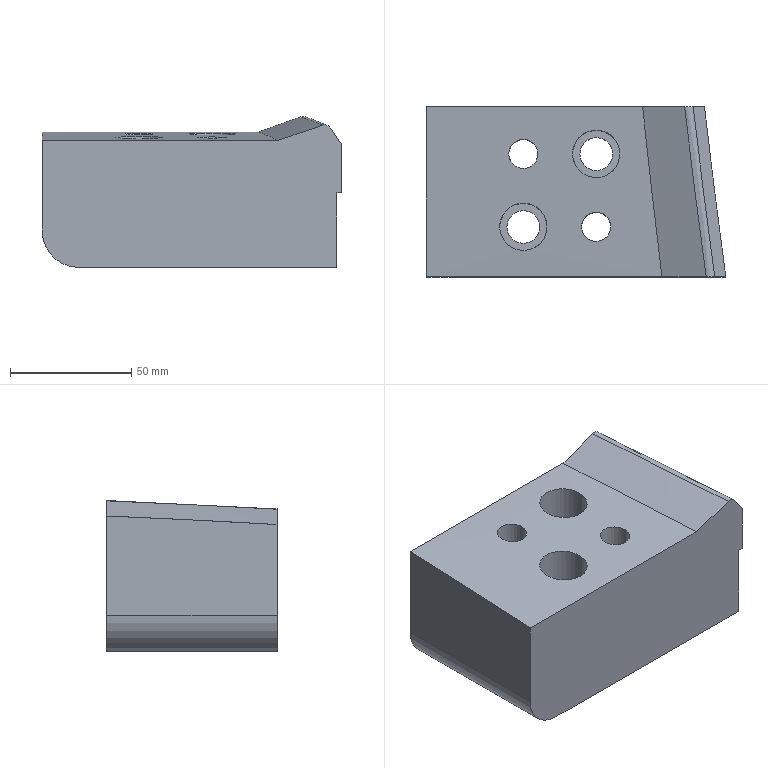Part | NX | features MAIN_BODY 2 | 1 solid | 20 faces | box 123.323 x 70 x 62.141 mm | volume 406291 mm3 | spline 7 | cylinder 7 | plane 6 | commonest cylinder face diameters 12 x2 13.5 x2 19.5 x2 30 x1
STEP:
#1=CARTESIAN_POINT('',(-841.75,-399.358,-90.));
#2=VERTEX_POINT('',#1);
#3=CARTESIAN_POINT('',(-835.,-399.358,-90.));
#4=DIRECTION('',(-0.000000341,0.00000017,-1.));
#5=DIRECTION('',(-1.,0.,0.000000341));
#6=AXIS2_PLACEMENT_3D('',#3,#4,#5);
#7=CIRCLE('',#6,6.75);
#8=EDGE_CURVE('',#2,#2,#7,.T.);
#9=ORIENTED_EDGE('',*,*,#8,.F.);
#10=EDGE_LOOP('',(#9));
#11=FACE_BOUND('',#10,.T.);
#12=CARTESIAN_POINT('',(-841.,-369.358,-90.));
#13=VERTEX_POINT('',#12);
#14=CARTESIAN_POINT('',(-835.,-369.358,-90.));
#15=DIRECTION('',(-0.000000341,0.00000017,-1.));
#16=DIRECTION('',(-1.,0.,0.000000341));
#17=AXIS2_PLACEMENT_3D('',#14,#15,#16);
#18=CIRCLE('',#17,6.);
#19=EDGE_CURVE('',#13,#13,#18,.T.);
#20=ORIENTED_EDGE('',*,*,#19,.F.);
#21=EDGE_LOOP('',(#20));
#22=FACE_BOUND('',#21,.T.);
#23=CARTESIAN_POINT('',(-811.75,-369.358,-90.));
#24=VERTEX_POINT('',#23);
#25=CARTESIAN_POINT('',(-805.,-369.358,-90.));
#26=DIRECTION('',(-0.000000341,0.00000017,-1.));
#27=DIRECTION('',(-1.,0.,0.000000341));
#28=AXIS2_PLACEMENT_3D('',#25,#26,#27);
#29=CIRCLE('',#28,6.75);
#30=EDGE_CURVE('',#24,#24,#29,.T.);
#31=ORIENTED_EDGE('',*,*,#30,.F.);
#32=EDGE_LOOP('',(#31));
#33=FACE_BOUND('',#32,.T.);
#34=CARTESIAN_POINT('',(-811.,-399.358,-90.));
#35=VERTEX_POINT('',#34);
#36=CARTESIAN_POINT('',(-805.,-399.358,-90.));
#37=DIRECTION('',(-0.000000341,0.00000017,-1.));
#38=DIRECTION('',(-1.,0.,0.000000341));
#39=AXIS2_PLACEMENT_3D('',#36,#37,#38);
#40=CIRCLE('',#39,6.);
#41=EDGE_CURVE('',#35,#35,#40,.T.);
#42=ORIENTED_EDGE('',*,*,#41,.F.);
#43=EDGE_LOOP('',(#42));
#44=FACE_BOUND('',#43,.T.);
#45=CARTESIAN_POINT('',(-860.,-350.,-90.));
#46=VERTEX_POINT('',#45);
#47=CARTESIAN_POINT('',(-762.48,-350.,-90.));
#48=VERTEX_POINT('',#47);
#49=CARTESIAN_POINT('',(-0.00003074,-350.,-90.));
#50=DIRECTION('',(-1.,0.,0.000000341));
#51=VECTOR('',#50,1000.);
#52=LINE('',#49,#51);
#53=EDGE_CURVE('',#46,#48,#52,.F.);
#54=ORIENTED_EDGE('',*,*,#53,.T.);
#55=CARTESIAN_POINT('',(-753.694,-420.,-90.));
#56=VERTEX_POINT('',#55);
#57=CARTESIAN_POINT('',(-753.694,-420.,-90.));
#58=CARTESIAN_POINT('',(-755.213,-408.34,-90.));
#59=CARTESIAN_POINT('',(-758.313,-385.028,-90.));
#60=CARTESIAN_POINT('',(-761.09,-361.676,-90.));
#61=CARTESIAN_POINT('',(-762.48,-350.,-90.));
#62=B_SPLINE_CURVE_WITH_KNOTS('',3,(#57,#58,#59,#60,#61),.UNSPECIFIED.,.F.,.F.,(4,1,4),(0.,0.03528,0.07055),.UNSPECIFIED.);
#63=EDGE_CURVE('',#56,#48,#62,.T.);
#64=ORIENTED_EDGE('',*,*,#63,.F.);
#65=CARTESIAN_POINT('',(-860.,-420.,-90.));
#66=VERTEX_POINT('',#65);
#67=CARTESIAN_POINT('',(-0.00003074,-420.,-90.));
#68=DIRECTION('',(-1.,0.,0.000000341));
#69=VECTOR('',#68,1000.);
#70=LINE('',#67,#69);
#71=EDGE_CURVE('',#66,#56,#70,.F.);
#72=ORIENTED_EDGE('',*,*,#71,.F.);
#73=CARTESIAN_POINT('',(-860.,-739.25,-90.));
#74=DIRECTION('',(0.000000011,1.,0.00000017));
#75=VECTOR('',#74,1000.);
#76=LINE('',#73,#75);
#77=EDGE_CURVE('',#46,#66,#76,.F.);
#78=ORIENTED_EDGE('',*,*,#77,.F.);
#79=EDGE_LOOP('',(#54,#64,#72,#78));
#80=FACE_BOUND('',#79,.T.);
#81=CARTESIAN_POINT('',(-780.,-1058.533,-90.));
#82=DIRECTION('',(-0.000000341,0.00000017,-1.));
#83=DIRECTION('',(-0.000000011,-1.,-0.00000017));
#84=AXIS2_PLACEMENT_3D('',#81,#82,#83);
#85=PLANE('',#84);
#86=ADVANCED_FACE('',(#11,#22,#33,#44,#80),#85,.T.);
#87=CARTESIAN_POINT('',(-751.677,-420.,-39.281));
#88=VERTEX_POINT('',#87);
#89=CARTESIAN_POINT('',(-756.237,-420.,-32.638));
#90=VERTEX_POINT('',#89);
#91=CARTESIAN_POINT('',(-751.677,-420.,-39.281));
#92=CARTESIAN_POINT('',(-753.197,-420.,-37.066));
#93=CARTESIAN_POINT('',(-754.717,-420.,-34.852));
#94=CARTESIAN_POINT('',(-756.237,-420.,-32.638));
#95=B_SPLINE_CURVE_WITH_KNOTS('',3,(#91,#92,#93,#94),.UNSPECIFIED.,.F.,.F.,(4,4),(0.,0.008057),.UNSPECIFIED.);
#96=EDGE_CURVE('',#88,#90,#95,.T.);
#97=ORIENTED_EDGE('',*,*,#96,.T.);
#98=CARTESIAN_POINT('',(-759.743,-420.,-31.477));
#99=VERTEX_POINT('',#98);
#100=CARTESIAN_POINT('',(-756.237,-420.,-32.638));
#101=CARTESIAN_POINT('',(-756.992,-420.,-31.539));
#102=CARTESIAN_POINT('',(-758.481,-420.,-31.044));
#103=CARTESIAN_POINT('',(-759.743,-420.,-31.477));
#104=B_SPLINE_CURVE_WITH_KNOTS('',3,(#100,#101,#102,#103),.UNSPECIFIED.,.F.,.F.,(4,4),(0.,0.003944),.UNSPECIFIED.);
#105=EDGE_CURVE('',#90,#99,#104,.T.);
#106=ORIENTED_EDGE('',*,*,#105,.T.);
#107=CARTESIAN_POINT('',(-777.971,-420.,-37.736));
#108=VERTEX_POINT('',#107);
#109=CARTESIAN_POINT('',(-759.743,-420.,-31.477));
#110=CARTESIAN_POINT('',(-765.819,-420.,-33.563));
#111=CARTESIAN_POINT('',(-771.895,-420.,-35.649));
#112=CARTESIAN_POINT('',(-777.971,-420.,-37.736));
#113=B_SPLINE_CURVE_WITH_KNOTS('',3,(#109,#110,#111,#112),.UNSPECIFIED.,.F.,.F.,(4,4),(0.,0.01927),.UNSPECIFIED.);
#114=EDGE_CURVE('',#99,#108,#113,.T.);
#115=ORIENTED_EDGE('',*,*,#114,.T.);
#116=CARTESIAN_POINT('',(-875.,-420.,-37.736));
#117=VERTEX_POINT('',#116);
#118=CARTESIAN_POINT('',(-875.,-420.,-37.736));
#119=CARTESIAN_POINT('',(-842.657,-420.,-37.736));
#120=CARTESIAN_POINT('',(-810.314,-420.,-37.736));
#121=CARTESIAN_POINT('',(-777.971,-420.,-37.736));
#122=B_SPLINE_CURVE_WITH_KNOTS('',3,(#118,#119,#120,#121),.UNSPECIFIED.,.F.,.F.,(4,4),(-0.01,0.08703),.UNSPECIFIED.);
#123=EDGE_CURVE('',#117,#108,#122,.T.);
#124=ORIENTED_EDGE('',*,*,#123,.F.);
#125=CARTESIAN_POINT('',(-875.,-420.,-75.));
#126=VERTEX_POINT('',#125);
#127=CARTESIAN_POINT('',(-875.,-420.,0.0002989));
#128=DIRECTION('',(0.000000341,0.,1.));
#129=VECTOR('',#128,1000.);
#130=LINE('',#127,#129);
#131=EDGE_CURVE('',#126,#117,#130,.T.);
#132=ORIENTED_EDGE('',*,*,#131,.F.);
#133=CARTESIAN_POINT('',(-860.,-420.,-75.));
#134=DIRECTION('',(0.,1.,0.));
#135=DIRECTION('',(0.,0.,1.));
#136=AXIS2_PLACEMENT_3D('',#133,#134,#135);
#137=CIRCLE('',#136,15.);
#138=EDGE_CURVE('',#66,#126,#137,.T.);
#139=ORIENTED_EDGE('',*,*,#138,.F.);
#140=ORIENTED_EDGE('',*,*,#71,.T.);
#141=CARTESIAN_POINT('',(-753.694,-420.,-59.267));
#142=VERTEX_POINT('',#141);
#143=CARTESIAN_POINT('',(-753.694,-420.,-74.594));
#144=DIRECTION('',(0.,0.,1.));
#145=VECTOR('',#144,1000.);
#146=LINE('',#143,#145);
#147=EDGE_CURVE('',#142,#56,#146,.F.);
#148=ORIENTED_EDGE('',*,*,#147,.F.);
#149=CARTESIAN_POINT('',(-751.677,-420.,-59.281));
#150=VERTEX_POINT('',#149);
#151=CARTESIAN_POINT('',(-753.694,-420.,-59.267));
#152=CARTESIAN_POINT('',(-753.022,-420.,-59.272));
#153=CARTESIAN_POINT('',(-752.35,-420.,-59.276));
#154=CARTESIAN_POINT('',(-751.677,-420.,-59.281));
#155=B_SPLINE_CURVE_WITH_KNOTS('',3,(#151,#152,#153,#154),.UNSPECIFIED.,.F.,.F.,(4,4),(0.,0.002017),.UNSPECIFIED.);
#156=EDGE_CURVE('',#142,#150,#155,.T.);
#157=ORIENTED_EDGE('',*,*,#156,.T.);
#158=CARTESIAN_POINT('',(-751.677,-420.,-49.201));
#159=DIRECTION('',(0.,0.,1.));
#160=VECTOR('',#159,1000.);
#161=LINE('',#158,#160);
#162=EDGE_CURVE('',#88,#150,#161,.F.);
#163=ORIENTED_EDGE('',*,*,#162,.F.);
#164=EDGE_LOOP('',(#97,#106,#115,#124,#132,#139,#140,#148,#157,#163));
#165=FACE_BOUND('',#164,.T.);
#166=CARTESIAN_POINT('',(0.,-420.,0.));
#167=DIRECTION('',(0.,1.,0.));
#168=DIRECTION('',(0.,0.,1.));
#169=AXIS2_PLACEMENT_3D('',#166,#167,#168);
#170=PLANE('',#169);
#171=ADVANCED_FACE('',(#165),#170,.F.);
#172=CARTESIAN_POINT('',(-760.466,-350.,-35.75));
#173=VERTEX_POINT('',#172);
#174=CARTESIAN_POINT('',(-760.466,-350.,-55.75));
#175=VERTEX_POINT('',#174);
#176=CARTESIAN_POINT('',(-760.466,-350.,-45.819));
#177=DIRECTION('',(0.,0.,1.));
#178=VECTOR('',#177,1000.);
#179=LINE('',#176,#178);
#180=EDGE_CURVE('',#173,#175,#179,.F.);
#181=ORIENTED_EDGE('',*,*,#180,.F.);
#182=CARTESIAN_POINT('',(-760.466,-350.,-35.75));
#183=CARTESIAN_POINT('',(-759.076,-361.679,-36.278));
#184=CARTESIAN_POINT('',(-756.296,-385.037,-37.348));
#185=CARTESIAN_POINT('',(-753.196,-408.342,-38.648));
#186=CARTESIAN_POINT('',(-751.677,-420.,-39.281));
#187=B_SPLINE_CURVE_WITH_KNOTS('',3,(#182,#183,#184,#185,#186),.UNSPECIFIED.,.F.,.F.,(4,1,4),(-0.001545,0.03377,0.06909),.UNSPECIFIED.);
#188=EDGE_CURVE('',#173,#88,#187,.T.);
#189=ORIENTED_EDGE('',*,*,#188,.T.);
#190=ORIENTED_EDGE('',*,*,#162,.T.);
#191=CARTESIAN_POINT('',(-751.677,-420.,-59.281));
#192=CARTESIAN_POINT('',(-753.196,-408.342,-58.648));
#193=CARTESIAN_POINT('',(-756.296,-385.037,-57.348));
#194=CARTESIAN_POINT('',(-759.076,-361.679,-56.278));
#195=CARTESIAN_POINT('',(-760.466,-350.,-55.75));
#196=B_SPLINE_CURVE_WITH_KNOTS('',3,(#191,#192,#193,#194,#195),.UNSPECIFIED.,.F.,.F.,(4,1,4),(-0.001482,0.03384,0.06916),.UNSPECIFIED.);
#197=EDGE_CURVE('',#150,#175,#196,.T.);
#198=ORIENTED_EDGE('',*,*,#197,.T.);
#199=EDGE_LOOP('',(#181,#189,#190,#198));
#200=FACE_BOUND('',#199,.T.);
#201=CARTESIAN_POINT('',(-760.466,-350.,-55.89));
#202=CARTESIAN_POINT('',(-760.466,-350.,-35.604));
#203=CARTESIAN_POINT('',(-759.076,-361.678,-56.437));
#204=CARTESIAN_POINT('',(-759.076,-361.678,-36.15));
#205=CARTESIAN_POINT('',(-756.296,-385.034,-57.531));
#206=CARTESIAN_POINT('',(-756.296,-385.034,-37.244));
#207=CARTESIAN_POINT('',(-753.196,-408.342,-58.788));
#208=CARTESIAN_POINT('',(-753.196,-408.342,-38.501));
#209=CARTESIAN_POINT('',(-751.677,-420.,-59.401));
#210=CARTESIAN_POINT('',(-751.677,-420.,-39.114));
#211=B_SPLINE_SURFACE_WITH_KNOTS('',3,1,((#201,#202),(#203,#204),(#205,#206),(#207,#208),(#209,#210)),.SURF_OF_LINEAR_EXTRUSION.,.F.,.F.,.F.,(4,1,4),(2,2),(-0.4271,0.68,1.787),(0.,1.),.UNSPECIFIED.);
#212=ADVANCED_FACE('',(#200),#211,.F.);
#213=ORIENTED_EDGE('',*,*,#131,.T.);
#214=CARTESIAN_POINT('',(-875.,-350.,-34.252));
#215=VERTEX_POINT('',#214);
#216=CARTESIAN_POINT('',(-875.,-350.,-34.252));
#217=CARTESIAN_POINT('',(-875.,-373.342,-35.241));
#218=CARTESIAN_POINT('',(-875.,-396.676,-36.394));
#219=CARTESIAN_POINT('',(-875.,-420.,-37.736));
#220=B_SPLINE_CURVE_WITH_KNOTS('',3,(#216,#217,#218,#219),.UNSPECIFIED.,.F.,.F.,(4,4),(0.2837,0.3538),.UNSPECIFIED.);
#221=EDGE_CURVE('',#117,#215,#220,.F.);
#222=ORIENTED_EDGE('',*,*,#221,.T.);
#223=CARTESIAN_POINT('',(-875.,-350.,-75.));
#224=VERTEX_POINT('',#223);
#225=CARTESIAN_POINT('',(-875.,-350.,0.0002989));
#226=DIRECTION('',(0.000000341,0.,1.));
#227=VECTOR('',#226,1000.);
#228=LINE('',#225,#227);
#229=EDGE_CURVE('',#224,#215,#228,.T.);
#230=ORIENTED_EDGE('',*,*,#229,.F.);
#231=CARTESIAN_POINT('',(-875.,-739.25,-75.));
#232=DIRECTION('',(0.000000011,1.,0.00000017));
#233=VECTOR('',#232,1000.);
#234=LINE('',#231,#233);
#235=EDGE_CURVE('',#126,#224,#234,.T.);
#236=ORIENTED_EDGE('',*,*,#235,.F.);
#237=EDGE_LOOP('',(#213,#222,#230,#236));
#238=FACE_BOUND('',#237,.T.);
#239=CARTESIAN_POINT('',(-875.,-739.25,-90.));
#240=DIRECTION('',(-1.,0.000000011,0.000000341));
#241=DIRECTION('',(-0.000000341,0.00000017,-1.));
#242=AXIS2_PLACEMENT_3D('',#239,#240,#241);
#243=PLANE('',#242);
#244=ADVANCED_FACE('',(#238),#243,.T.);
#245=CARTESIAN_POINT('',(-802.615,-378.812,-35.56));
#246=VERTEX_POINT('',#245);
#247=CARTESIAN_POINT('',(-810.554,-378.63,-35.551));
#248=CARTESIAN_POINT('',(-802.353,-379.838,-35.61));
#249=CARTESIAN_POINT('',(-795.722,-374.891,-35.371));
#250=CARTESIAN_POINT('',(-794.523,-366.727,-34.987));
#251=CARTESIAN_POINT('',(-799.45,-360.085,-34.688));
#252=CARTESIAN_POINT('',(-807.643,-358.881,-34.635));
#253=CARTESIAN_POINT('',(-814.27,-363.813,-34.854));
#254=CARTESIAN_POINT('',(-815.479,-371.987,-35.232));
#255=CARTESIAN_POINT('',(-810.554,-378.63,-35.551));
#256=CARTESIAN_POINT('',(-802.353,-379.838,-35.61));
#257=CARTESIAN_POINT('',(-795.722,-374.891,-35.371));
#258=B_SPLINE_CURVE_WITH_KNOTS('',3,(#247,#248,#249,#250,#251,#252,#253,#254,#255,#256,#257),.UNSPECIFIED.,.T.,.F.,(1,1,1,1,1,1,1,1,1,1,1,1,1,1,1),(-0.02287,-0.01525,-0.007624,0.,0.007624,0.01525,0.02287,0.0305,0.03812,0.04574,0.05337,0.06099,0.06862,0.07624,0.08386),.UNSPECIFIED.);
#259=EDGE_CURVE('',#246,#246,#258,.T.);
#260=ORIENTED_EDGE('',*,*,#259,.F.);
#261=EDGE_LOOP('',(#260));
#262=FACE_BOUND('',#261,.T.);
#263=CARTESIAN_POINT('',(-806.104,-405.256,-36.91));
#264=VERTEX_POINT('',#263);
#265=CARTESIAN_POINT('',(-810.492,-403.108,-36.793));
#266=CARTESIAN_POINT('',(-806.223,-405.897,-36.944));
#267=CARTESIAN_POINT('',(-801.239,-404.841,-36.887));
#268=CARTESIAN_POINT('',(-798.467,-400.584,-36.658));
#269=CARTESIAN_POINT('',(-799.51,-395.607,-36.398));
#270=CARTESIAN_POINT('',(-803.775,-392.823,-36.256));
#271=CARTESIAN_POINT('',(-808.753,-393.871,-36.309));
#272=CARTESIAN_POINT('',(-811.534,-398.131,-36.529));
#273=CARTESIAN_POINT('',(-810.492,-403.108,-36.793));
#274=CARTESIAN_POINT('',(-806.223,-405.897,-36.944));
#275=CARTESIAN_POINT('',(-801.239,-404.841,-36.887));
#276=B_SPLINE_CURVE_WITH_KNOTS('',3,(#265,#266,#267,#268,#269,#270,#271,#272,#273,#274,#275),.UNSPECIFIED.,.T.,.F.,(1,1,1,1,1,1,1,1,1,1,1,1,1,1,1),(-0.01408,-0.009385,-0.004692,0.,0.004692,0.009385,0.01408,0.01877,0.02346,0.02815,0.03285,0.03754,0.04223,0.04692,0.05162),.UNSPECIFIED.);
#277=EDGE_CURVE('',#264,#264,#276,.T.);
#278=ORIENTED_EDGE('',*,*,#277,.F.);
#279=EDGE_LOOP('',(#278));
#280=FACE_BOUND('',#279,.T.);
#281=CARTESIAN_POINT('',(-785.933,-350.,-34.252));
#282=VERTEX_POINT('',#281);
#283=CARTESIAN_POINT('',(-875.,-350.,-34.252));
#284=CARTESIAN_POINT('',(-845.311,-350.,-34.252));
#285=CARTESIAN_POINT('',(-815.622,-350.,-34.252));
#286=CARTESIAN_POINT('',(-785.933,-350.,-34.252));
#287=B_SPLINE_CURVE_WITH_KNOTS('',3,(#283,#284,#285,#286),.UNSPECIFIED.,.F.,.F.,(4,4),(-0.01,0.07907),.UNSPECIFIED.);
#288=EDGE_CURVE('',#215,#282,#287,.T.);
#289=ORIENTED_EDGE('',*,*,#288,.F.);
#290=ORIENTED_EDGE('',*,*,#221,.F.);
#291=ORIENTED_EDGE('',*,*,#123,.T.);
#292=CARTESIAN_POINT('',(-777.971,-420.,-37.736));
#293=CARTESIAN_POINT('',(-780.789,-396.695,-36.395));
#294=CARTESIAN_POINT('',(-783.443,-373.36,-35.242));
#295=CARTESIAN_POINT('',(-785.933,-350.,-34.252));
#296=B_SPLINE_CURVE_WITH_KNOTS('',3,(#292,#293,#294,#295),.UNSPECIFIED.,.F.,.F.,(4,4),(0.1656,0.2359),.UNSPECIFIED.);
#297=EDGE_CURVE('',#108,#282,#296,.T.);
#298=ORIENTED_EDGE('',*,*,#297,.T.);
#299=EDGE_LOOP('',(#289,#290,#291,#298));
#300=FACE_BOUND('',#299,.T.);
#301=CARTESIAN_POINT('',(-837.117,-374.973,-35.376));
#302=VERTEX_POINT('',#301);
#303=CARTESIAN_POINT('',(-841.061,-372.092,-35.239));
#304=CARTESIAN_POINT('',(-837.346,-375.582,-35.405));
#305=CARTESIAN_POINT('',(-832.255,-375.414,-35.397));
#306=CARTESIAN_POINT('',(-828.781,-371.706,-35.22));
#307=CARTESIAN_POINT('',(-828.94,-366.622,-34.983));
#308=CARTESIAN_POINT('',(-832.652,-363.137,-34.825));
#309=CARTESIAN_POINT('',(-837.736,-363.299,-34.832));
#310=CARTESIAN_POINT('',(-841.22,-367.009,-35.001));
#311=CARTESIAN_POINT('',(-841.061,-372.092,-35.239));
#312=CARTESIAN_POINT('',(-837.346,-375.582,-35.405));
#313=CARTESIAN_POINT('',(-832.255,-375.414,-35.397));
#314=B_SPLINE_CURVE_WITH_KNOTS('',3,(#303,#304,#305,#306,#307,#308,#309,#310,#311,#312,#313),.UNSPECIFIED.,.T.,.F.,(1,1,1,1,1,1,1,1,1,1,1,1,1,1,1),(-0.01408,-0.009384,-0.004692,0.,0.004692,0.009384,0.01408,0.01877,0.02346,0.02815,0.03284,0.03753,0.04223,0.04692,0.05161),.UNSPECIFIED.);
#315=EDGE_CURVE('',#302,#302,#314,.T.);
#316=ORIENTED_EDGE('',*,*,#315,.F.);
#317=EDGE_LOOP('',(#316));
#318=FACE_BOUND('',#317,.T.);
#319=CARTESIAN_POINT('',(-844.701,-400.333,-36.646));
#320=VERTEX_POINT('',#319);
#321=CARTESIAN_POINT('',(-843.364,-392.516,-36.238));
#322=CARTESIAN_POINT('',(-845.751,-400.44,-36.648));
#323=CARTESIAN_POINT('',(-841.839,-407.721,-37.043));
#324=CARTESIAN_POINT('',(-833.927,-410.11,-37.176));
#325=CARTESIAN_POINT('',(-826.634,-406.198,-36.959));
#326=CARTESIAN_POINT('',(-824.252,-398.282,-36.535));
#327=CARTESIAN_POINT('',(-828.148,-391.005,-36.162));
#328=CARTESIAN_POINT('',(-836.069,-388.604,-36.043));
#329=CARTESIAN_POINT('',(-843.364,-392.516,-36.238));
#330=CARTESIAN_POINT('',(-845.751,-400.44,-36.648));
#331=CARTESIAN_POINT('',(-841.839,-407.721,-37.043));
#332=B_SPLINE_CURVE_WITH_KNOTS('',3,(#321,#322,#323,#324,#325,#326,#327,#328,#329,#330,#331),.UNSPECIFIED.,.T.,.F.,(1,1,1,1,1,1,1,1,1,1,1,1,1,1,1),(-0.02288,-0.01525,-0.007625,0.,0.007625,0.01525,0.02288,0.0305,0.03813,0.04575,0.05338,0.061,0.06863,0.07625,0.08388),.UNSPECIFIED.);
#333=EDGE_CURVE('',#320,#320,#332,.T.);
#334=ORIENTED_EDGE('',*,*,#333,.F.);
#335=EDGE_LOOP('',(#334));
#336=FACE_BOUND('',#335,.T.);
#337=CARTESIAN_POINT('',(-875.566,-420.159,-37.746));
#338=CARTESIAN_POINT('',(-776.547,-420.159,-37.746));
#339=CARTESIAN_POINT('',(-877.1,-408.39,-37.068));
#340=CARTESIAN_POINT('',(-778.081,-408.39,-37.068));
#341=CARTESIAN_POINT('',(-880.224,-384.914,-35.815));
#342=CARTESIAN_POINT('',(-781.205,-384.914,-35.815));
#343=CARTESIAN_POINT('',(-883.011,-361.373,-34.734));
#344=CARTESIAN_POINT('',(-783.992,-361.373,-34.734));
#345=CARTESIAN_POINT('',(-884.415,-349.579,-34.234));
#346=CARTESIAN_POINT('',(-785.396,-349.579,-34.234));
#347=B_SPLINE_SURFACE_WITH_KNOTS('',3,1,((#337,#338),(#339,#340),(#341,#342),(#343,#344),(#345,#346)),.SURF_OF_LINEAR_EXTRUSION.,.F.,.F.,.F.,(4,1,4),(2,2),(-0.0303,0.4972,1.025),(0.,1.),.UNSPECIFIED.);
#348=ADVANCED_FACE('',(#262,#280,#300,#318,#336),#347,.F.);
#349=CARTESIAN_POINT('',(-768.637,-350.,-28.029));
#350=VERTEX_POINT('',#349);
#351=CARTESIAN_POINT('',(-768.637,-350.,-28.029));
#352=CARTESIAN_POINT('',(-774.403,-350.,-30.103));
#353=CARTESIAN_POINT('',(-780.168,-350.,-32.177));
#354=CARTESIAN_POINT('',(-785.933,-350.,-34.252));
#355=B_SPLINE_CURVE_WITH_KNOTS('',3,(#351,#352,#353,#354),.UNSPECIFIED.,.F.,.F.,(4,4),(0.,0.01838),.UNSPECIFIED.);
#356=EDGE_CURVE('',#350,#282,#355,.T.);
#357=ORIENTED_EDGE('',*,*,#356,.F.);
#358=CARTESIAN_POINT('',(-765.126,-350.,-29.138));
#359=VERTEX_POINT('',#358);
#360=CARTESIAN_POINT('',(-768.637,-350.,-28.029));
#361=CARTESIAN_POINT('',(-767.385,-350.,-27.578));
#362=CARTESIAN_POINT('',(-765.892,-350.,-28.05));
#363=CARTESIAN_POINT('',(-765.126,-350.,-29.138));
#364=B_SPLINE_CURVE_WITH_KNOTS('',3,(#360,#361,#362,#363),.UNSPECIFIED.,.F.,.F.,(4,4),(0.,0.003934),.UNSPECIFIED.);
#365=EDGE_CURVE('',#350,#359,#364,.T.);
#366=ORIENTED_EDGE('',*,*,#365,.T.);
#367=CARTESIAN_POINT('',(-765.126,-350.,-29.138));
#368=CARTESIAN_POINT('',(-763.572,-350.,-31.342));
#369=CARTESIAN_POINT('',(-762.019,-350.,-33.546));
#370=CARTESIAN_POINT('',(-760.466,-350.,-35.75));
#371=B_SPLINE_CURVE_WITH_KNOTS('',3,(#367,#368,#369,#370),.UNSPECIFIED.,.F.,.F.,(4,4),(0.,0.008089),.UNSPECIFIED.);
#372=EDGE_CURVE('',#359,#173,#371,.T.);
#373=ORIENTED_EDGE('',*,*,#372,.T.);
#374=ORIENTED_EDGE('',*,*,#180,.T.);
#375=CARTESIAN_POINT('',(-762.48,-350.,-55.739));
#376=VERTEX_POINT('',#375);
#377=CARTESIAN_POINT('',(-760.466,-350.,-55.75));
#378=CARTESIAN_POINT('',(-761.137,-350.,-55.746));
#379=CARTESIAN_POINT('',(-761.808,-350.,-55.743));
#380=CARTESIAN_POINT('',(-762.48,-350.,-55.739));
#381=B_SPLINE_CURVE_WITH_KNOTS('',3,(#377,#378,#379,#380),.UNSPECIFIED.,.F.,.F.,(4,4),(0.,0.002014),.UNSPECIFIED.);
#382=EDGE_CURVE('',#175,#376,#381,.T.);
#383=ORIENTED_EDGE('',*,*,#382,.T.);
#384=CARTESIAN_POINT('',(-762.48,-350.,-72.904));
#385=DIRECTION('',(0.,0.,1.));
#386=VECTOR('',#385,1000.);
#387=LINE('',#384,#386);
#388=EDGE_CURVE('',#376,#48,#387,.F.);
#389=ORIENTED_EDGE('',*,*,#388,.T.);
#390=ORIENTED_EDGE('',*,*,#53,.F.);
#391=CARTESIAN_POINT('',(-860.,-350.,-75.));
#392=DIRECTION('',(0.,1.,0.));
#393=DIRECTION('',(0.,0.,1.));
#394=AXIS2_PLACEMENT_3D('',#391,#392,#393);
#395=CIRCLE('',#394,15.);
#396=EDGE_CURVE('',#224,#46,#395,.F.);
#397=ORIENTED_EDGE('',*,*,#396,.F.);
#398=ORIENTED_EDGE('',*,*,#229,.T.);
#399=ORIENTED_EDGE('',*,*,#288,.T.);
#400=EDGE_LOOP('',(#357,#366,#373,#374,#383,#389,#390,#397,#398,#399));
#401=FACE_BOUND('',#400,.T.);
#402=CARTESIAN_POINT('',(0.,-350.,0.));
#403=DIRECTION('',(0.,1.,0.));
#404=DIRECTION('',(0.,0.,1.));
#405=AXIS2_PLACEMENT_3D('',#402,#403,#404);
#406=PLANE('',#405);
#407=ADVANCED_FACE('',(#401),#406,.T.);
#408=CARTESIAN_POINT('',(-844.75,-399.358,-80.));
#409=VERTEX_POINT('',#408);
#410=CARTESIAN_POINT('',(-835.,-399.358,-80.));
#411=DIRECTION('',(0.000000341,-0.00000017,1.));
#412=DIRECTION('',(-1.,0.,0.000000341));
#413=AXIS2_PLACEMENT_3D('',#410,#411,#412);
#414=CIRCLE('',#413,9.75);
#415=EDGE_CURVE('',#409,#409,#414,.F.);
#416=ORIENTED_EDGE('',*,*,#415,.T.);
#417=EDGE_LOOP('',(#416));
#418=FACE_BOUND('',#417,.T.);
#419=ORIENTED_EDGE('',*,*,#333,.T.);
#420=EDGE_LOOP('',(#419));
#421=FACE_BOUND('',#420,.T.);
#422=CARTESIAN_POINT('',(-835.,-399.358,-70.));
#423=DIRECTION('',(0.000000341,-0.00000017,1.));
#424=DIRECTION('',(0.000000011,1.,0.00000017));
#425=AXIS2_PLACEMENT_3D('',#422,#423,#424);
#426=CYLINDRICAL_SURFACE('',#425,9.75);
#427=ADVANCED_FACE('',(#418,#421),#426,.F.);
#428=CARTESIAN_POINT('',(-841.75,-399.358,-80.));
#429=VERTEX_POINT('',#428);
#430=CARTESIAN_POINT('',(-835.,-399.358,-80.));
#431=DIRECTION('',(0.000000341,-0.00000017,1.));
#432=DIRECTION('',(-1.,0.,0.000000341));
#433=AXIS2_PLACEMENT_3D('',#430,#431,#432);
#434=CIRCLE('',#433,6.75);
#435=EDGE_CURVE('',#429,#429,#434,.F.);
#436=ORIENTED_EDGE('',*,*,#435,.F.);
#437=EDGE_LOOP('',(#436));
#438=FACE_BOUND('',#437,.T.);
#439=ORIENTED_EDGE('',*,*,#8,.T.);
#440=EDGE_LOOP('',(#439));
#441=FACE_BOUND('',#440,.T.);
#442=CARTESIAN_POINT('',(-835.,-399.358,-90.));
#443=DIRECTION('',(0.000000341,-0.00000017,1.));
#444=DIRECTION('',(0.000000011,1.,0.00000017));
#445=AXIS2_PLACEMENT_3D('',#442,#443,#444);
#446=CYLINDRICAL_SURFACE('',#445,6.75);
#447=ADVANCED_FACE('',(#438,#441),#446,.F.);
#448=ORIENTED_EDGE('',*,*,#435,.T.);
#449=EDGE_LOOP('',(#448));
#450=FACE_BOUND('',#449,.T.);
#451=ORIENTED_EDGE('',*,*,#415,.F.);
#452=EDGE_LOOP('',(#451));
#453=FACE_BOUND('',#452,.T.);
#454=CARTESIAN_POINT('',(-835.,-399.358,-80.));
#455=DIRECTION('',(-0.000000341,0.00000017,-1.));
#456=DIRECTION('',(-0.000000011,-1.,-0.00000017));
#457=AXIS2_PLACEMENT_3D('',#454,#455,#456);
#458=PLANE('',#457);
#459=ADVANCED_FACE('',(#450,#453),#458,.F.);
#460=ORIENTED_EDGE('',*,*,#19,.T.);
#461=EDGE_LOOP('',(#460));
#462=FACE_BOUND('',#461,.T.);
#463=ORIENTED_EDGE('',*,*,#315,.T.);
#464=EDGE_LOOP('',(#463));
#465=FACE_BOUND('',#464,.T.);
#466=CARTESIAN_POINT('',(-835.,-369.358,-90.));
#467=DIRECTION('',(0.000000341,-0.00000017,1.));
#468=DIRECTION('',(0.000000011,1.,0.00000017));
#469=AXIS2_PLACEMENT_3D('',#466,#467,#468);
#470=CYLINDRICAL_SURFACE('',#469,6.);
#471=ADVANCED_FACE('',(#462,#465),#470,.F.);
#472=CARTESIAN_POINT('',(-814.75,-369.358,-80.));
#473=VERTEX_POINT('',#472);
#474=CARTESIAN_POINT('',(-805.,-369.358,-80.));
#475=DIRECTION('',(0.000000341,-0.00000017,1.));
#476=DIRECTION('',(-1.,0.,0.000000341));
#477=AXIS2_PLACEMENT_3D('',#474,#475,#476);
#478=CIRCLE('',#477,9.75);
#479=EDGE_CURVE('',#473,#473,#478,.F.);
#480=ORIENTED_EDGE('',*,*,#479,.T.);
#481=EDGE_LOOP('',(#480));
#482=FACE_BOUND('',#481,.T.);
#483=ORIENTED_EDGE('',*,*,#259,.T.);
#484=EDGE_LOOP('',(#483));
#485=FACE_BOUND('',#484,.T.);
#486=CARTESIAN_POINT('',(-805.,-369.358,-70.));
#487=DIRECTION('',(0.000000341,-0.00000017,1.));
#488=DIRECTION('',(0.000000011,1.,0.00000017));
#489=AXIS2_PLACEMENT_3D('',#486,#487,#488);
#490=CYLINDRICAL_SURFACE('',#489,9.75);
#491=ADVANCED_FACE('',(#482,#485),#490,.F.);
#492=CARTESIAN_POINT('',(-811.75,-369.358,-80.));
#493=VERTEX_POINT('',#492);
#494=CARTESIAN_POINT('',(-805.,-369.358,-80.));
#495=DIRECTION('',(0.000000341,-0.00000017,1.));
#496=DIRECTION('',(-1.,0.,0.000000341));
#497=AXIS2_PLACEMENT_3D('',#494,#495,#496);
#498=CIRCLE('',#497,6.75);
#499=EDGE_CURVE('',#493,#493,#498,.F.);
#500=ORIENTED_EDGE('',*,*,#499,.F.);
#501=EDGE_LOOP('',(#500));
#502=FACE_BOUND('',#501,.T.);
#503=ORIENTED_EDGE('',*,*,#30,.T.);
#504=EDGE_LOOP('',(#503));
#505=FACE_BOUND('',#504,.T.);
#506=CARTESIAN_POINT('',(-805.,-369.358,-90.));
#507=DIRECTION('',(0.000000341,-0.00000017,1.));
#508=DIRECTION('',(0.000000011,1.,0.00000017));
#509=AXIS2_PLACEMENT_3D('',#506,#507,#508);
#510=CYLINDRICAL_SURFACE('',#509,6.75);
#511=ADVANCED_FACE('',(#502,#505),#510,.F.);
#512=ORIENTED_EDGE('',*,*,#499,.T.);
#513=EDGE_LOOP('',(#512));
#514=FACE_BOUND('',#513,.T.);
#515=ORIENTED_EDGE('',*,*,#479,.F.);
#516=EDGE_LOOP('',(#515));
#517=FACE_BOUND('',#516,.T.);
#518=CARTESIAN_POINT('',(-805.,-369.358,-80.));
#519=DIRECTION('',(-0.000000341,0.00000017,-1.));
#520=DIRECTION('',(-0.000000011,-1.,-0.00000017));
#521=AXIS2_PLACEMENT_3D('',#518,#519,#520);
#522=PLANE('',#521);
#523=ADVANCED_FACE('',(#514,#517),#522,.F.);
#524=ORIENTED_EDGE('',*,*,#41,.T.);
#525=EDGE_LOOP('',(#524));
#526=FACE_BOUND('',#525,.T.);
#527=ORIENTED_EDGE('',*,*,#277,.T.);
#528=EDGE_LOOP('',(#527));
#529=FACE_BOUND('',#528,.T.);
#530=CARTESIAN_POINT('',(-805.,-399.358,-90.));
#531=DIRECTION('',(0.000000341,-0.00000017,1.));
#532=DIRECTION('',(0.000000011,1.,0.00000017));
#533=AXIS2_PLACEMENT_3D('',#530,#531,#532);
#534=CYLINDRICAL_SURFACE('',#533,6.);
#535=ADVANCED_FACE('',(#526,#529),#534,.F.);
#536=ORIENTED_EDGE('',*,*,#156,.F.);
#537=CARTESIAN_POINT('',(-753.694,-420.,-59.267));
#538=CARTESIAN_POINT('',(-755.213,-408.342,-58.634));
#539=CARTESIAN_POINT('',(-758.312,-385.037,-57.335));
#540=CARTESIAN_POINT('',(-761.09,-361.679,-56.267));
#541=CARTESIAN_POINT('',(-762.48,-350.,-55.739));
#542=B_SPLINE_CURVE_WITH_KNOTS('',3,(#537,#538,#539,#540,#541),.UNSPECIFIED.,.F.,.F.,(4,1,4),(-0.001482,0.03384,0.06916),.UNSPECIFIED.);
#543=EDGE_CURVE('',#142,#376,#542,.T.);
#544=ORIENTED_EDGE('',*,*,#543,.T.);
#545=ORIENTED_EDGE('',*,*,#382,.F.);
#546=ORIENTED_EDGE('',*,*,#197,.F.);
#547=EDGE_LOOP('',(#536,#544,#545,#546));
#548=FACE_BOUND('',#547,.T.);
#549=CARTESIAN_POINT('',(-751.658,-419.997,-59.281));
#550=CARTESIAN_POINT('',(-751.721,-419.508,-59.254));
#551=CARTESIAN_POINT('',(-751.785,-419.019,-59.228));
#552=CARTESIAN_POINT('',(-751.849,-418.53,-59.201));
#553=CARTESIAN_POINT('',(-753.303,-407.372,-58.596));
#554=CARTESIAN_POINT('',(-754.778,-396.218,-57.973));
#555=CARTESIAN_POINT('',(-757.606,-373.887,-56.841));
#556=CARTESIAN_POINT('',(-758.933,-362.709,-56.325));
#557=CARTESIAN_POINT('',(-760.264,-351.53,-55.819));
#558=CARTESIAN_POINT('',(-760.29,-351.307,-55.809));
#559=CARTESIAN_POINT('',(-760.317,-351.083,-55.799));
#560=CARTESIAN_POINT('',(-760.343,-350.86,-55.789));
#561=CARTESIAN_POINT('',(-760.387,-350.493,-55.772));
#562=CARTESIAN_POINT('',(-760.431,-350.127,-55.756));
#563=CARTESIAN_POINT('',(-760.474,-349.761,-55.739));
#564=CARTESIAN_POINT('',(-753.678,-420.261,-59.281));
#565=CARTESIAN_POINT('',(-753.742,-419.771,-59.254));
#566=CARTESIAN_POINT('',(-753.806,-419.282,-59.228));
#567=CARTESIAN_POINT('',(-753.869,-418.793,-59.201));
#568=CARTESIAN_POINT('',(-755.323,-407.637,-58.596));
#569=CARTESIAN_POINT('',(-756.799,-396.482,-57.973));
#570=CARTESIAN_POINT('',(-759.629,-374.135,-56.841));
#571=CARTESIAN_POINT('',(-760.957,-362.946,-56.325));
#572=CARTESIAN_POINT('',(-762.287,-351.771,-55.819));
#573=CARTESIAN_POINT('',(-762.313,-351.548,-55.809));
#574=CARTESIAN_POINT('',(-762.34,-351.324,-55.799));
#575=CARTESIAN_POINT('',(-762.367,-351.101,-55.789));
#576=CARTESIAN_POINT('',(-762.41,-350.734,-55.772));
#577=CARTESIAN_POINT('',(-762.454,-350.368,-55.756));
#578=CARTESIAN_POINT('',(-762.497,-350.002,-55.739));
#579=B_SPLINE_SURFACE_WITH_KNOTS('',1,3,((#549,#550,#551,#552,#553,#554,#555,#556,#557,#558,#559,#560,#561,#562,#563),(#564,#565,#566,#567,#568,#569,#570,#571,#572,#573,#574,#575,#576,#577,#578)),.RULED_SURF.,.F.,.F.,.F.,(2,2),(4,3,2,3,3,4),(0.498,0.7018),(-0.02192,0.,0.5,1.,1.01,1.026),.UNSPECIFIED.);
#580=ADVANCED_FACE('',(#548),#579,.T.);
#581=ORIENTED_EDGE('',*,*,#543,.F.);
#582=ORIENTED_EDGE('',*,*,#147,.T.);
#583=ORIENTED_EDGE('',*,*,#63,.T.);
#584=ORIENTED_EDGE('',*,*,#388,.F.);
#585=EDGE_LOOP('',(#581,#582,#583,#584));
#586=FACE_BOUND('',#585,.T.);
#587=CARTESIAN_POINT('',(-762.48,-350.,-90.206));
#588=CARTESIAN_POINT('',(-762.48,-350.,-55.506));
#589=CARTESIAN_POINT('',(-761.09,-361.674,-90.752));
#590=CARTESIAN_POINT('',(-761.09,-361.674,-56.053));
#591=CARTESIAN_POINT('',(-758.311,-385.042,-91.844));
#592=CARTESIAN_POINT('',(-758.311,-385.042,-57.145));
#593=CARTESIAN_POINT('',(-755.213,-408.345,-93.101));
#594=CARTESIAN_POINT('',(-755.213,-408.345,-58.402));
#595=CARTESIAN_POINT('',(-753.694,-420.,-93.714));
#596=CARTESIAN_POINT('',(-753.694,-420.,-59.014));
#597=B_SPLINE_SURFACE_WITH_KNOTS('',3,1,((#587,#588),(#589,#590),(#591,#592),(#593,#594),(#595,#596)),.SURF_OF_LINEAR_EXTRUSION.,.F.,.F.,.F.,(4,1,4),(2,2),(-0.4346,0.6722,1.779),(0.,1.),.UNSPECIFIED.);
#598=ADVANCED_FACE('',(#586),#597,.F.);
#599=ORIENTED_EDGE('',*,*,#138,.T.);
#600=ORIENTED_EDGE('',*,*,#235,.T.);
#601=ORIENTED_EDGE('',*,*,#396,.T.);
#602=ORIENTED_EDGE('',*,*,#77,.T.);
#603=EDGE_LOOP('',(#599,#600,#601,#602));
#604=FACE_BOUND('',#603,.T.);
#605=CARTESIAN_POINT('',(-860.,-739.25,-75.));
#606=DIRECTION('',(0.000000011,1.,0.00000017));
#607=DIRECTION('',(-0.000000341,0.00000017,-1.));
#608=AXIS2_PLACEMENT_3D('',#605,#606,#607);
#609=CYLINDRICAL_SURFACE('',#608,15.);
#610=ADVANCED_FACE('',(#604),#609,.T.);
#611=ORIENTED_EDGE('',*,*,#114,.F.);
#612=CARTESIAN_POINT('',(-759.743,-420.,-31.477));
#613=CARTESIAN_POINT('',(-762.888,-396.7,-30.139));
#614=CARTESIAN_POINT('',(-765.861,-373.365,-29.002));
#615=CARTESIAN_POINT('',(-768.637,-350.,-28.029));
#616=B_SPLINE_CURVE_WITH_KNOTS('',3,(#612,#613,#614,#615),.UNSPECIFIED.,.F.,.F.,(4,4),(-0.001483,0.06917),.UNSPECIFIED.);
#617=EDGE_CURVE('',#99,#350,#616,.T.);
#618=ORIENTED_EDGE('',*,*,#617,.T.);
#619=ORIENTED_EDGE('',*,*,#356,.T.);
#620=ORIENTED_EDGE('',*,*,#297,.F.);
#621=EDGE_LOOP('',(#611,#618,#619,#620));
#622=FACE_BOUND('',#621,.T.);
#623=CARTESIAN_POINT('',(-786.407,-349.588,-34.389));
#624=CARTESIAN_POINT('',(-780.371,-349.42,-32.203));
#625=CARTESIAN_POINT('',(-774.335,-349.252,-30.016));
#626=CARTESIAN_POINT('',(-768.299,-349.083,-27.83));
#627=CARTESIAN_POINT('',(-783.865,-373.411,-35.389));
#628=CARTESIAN_POINT('',(-777.801,-373.256,-33.222));
#629=CARTESIAN_POINT('',(-771.737,-373.101,-31.056));
#630=CARTESIAN_POINT('',(-765.672,-372.946,-28.89));
#631=CARTESIAN_POINT('',(-781.057,-397.131,-36.53));
#632=CARTESIAN_POINT('',(-774.96,-396.996,-34.387));
#633=CARTESIAN_POINT('',(-768.862,-396.86,-32.244));
#634=CARTESIAN_POINT('',(-762.765,-396.725,-30.101));
#635=CARTESIAN_POINT('',(-777.983,-420.75,-37.815));
#636=CARTESIAN_POINT('',(-771.848,-420.64,-35.698));
#637=CARTESIAN_POINT('',(-765.712,-420.53,-33.581));
#638=CARTESIAN_POINT('',(-759.577,-420.419,-31.464));
#639=B_SPLINE_SURFACE_WITH_KNOTS('',3,3,((#623,#624,#625,#626),(#627,#628,#629,#630),(#631,#632,#633,#634),(#635,#636,#637,#638)),.UNSPECIFIED.,.F.,.F.,.F.,(4,4),(4,4),(0.607,0.7329),(-0.6403,-0.1096),.UNSPECIFIED.);
#640=ADVANCED_FACE('',(#622),#639,.T.);
#641=ORIENTED_EDGE('',*,*,#372,.F.);
#642=CARTESIAN_POINT('',(-765.126,-350.,-29.138));
#643=CARTESIAN_POINT('',(-762.352,-373.365,-30.128));
#644=CARTESIAN_POINT('',(-759.378,-396.7,-31.282));
#645=CARTESIAN_POINT('',(-756.237,-420.,-32.638));
#646=B_SPLINE_CURVE_WITH_KNOTS('',3,(#642,#643,#644,#645),.UNSPECIFIED.,.F.,.F.,(4,4),(-0.001545,0.06911),.UNSPECIFIED.);
#647=EDGE_CURVE('',#359,#90,#646,.T.);
#648=ORIENTED_EDGE('',*,*,#647,.T.);
#649=ORIENTED_EDGE('',*,*,#96,.F.);
#650=ORIENTED_EDGE('',*,*,#188,.F.);
#651=EDGE_LOOP('',(#641,#648,#649,#650));
#652=FACE_BOUND('',#651,.T.);
#653=CARTESIAN_POINT('',(-740.602,-417.938,-55.704));
#654=CARTESIAN_POINT('',(-753.885,-420.924,-35.937));
#655=CARTESIAN_POINT('',(-760.317,-422.37,-26.365));
#656=CARTESIAN_POINT('',(-740.639,-417.646,-55.688));
#657=CARTESIAN_POINT('',(-753.923,-420.629,-35.922));
#658=CARTESIAN_POINT('',(-760.356,-422.074,-26.351));
#659=CARTESIAN_POINT('',(-740.676,-417.353,-55.673));
#660=CARTESIAN_POINT('',(-753.961,-420.334,-35.907));
#661=CARTESIAN_POINT('',(-760.395,-421.778,-26.336));
#662=CARTESIAN_POINT('',(-740.712,-417.061,-55.657));
#663=CARTESIAN_POINT('',(-754.,-420.039,-35.892));
#664=CARTESIAN_POINT('',(-760.433,-421.482,-26.321));
#665=CARTESIAN_POINT('',(-740.749,-416.768,-55.641));
#666=CARTESIAN_POINT('',(-754.038,-419.745,-35.877));
#667=CARTESIAN_POINT('',(-760.472,-421.186,-26.306));
#668=CARTESIAN_POINT('',(-740.786,-416.476,-55.625));
#669=CARTESIAN_POINT('',(-754.076,-419.45,-35.862));
#670=CARTESIAN_POINT('',(-760.511,-420.89,-26.291));
#671=CARTESIAN_POINT('',(-741.502,-410.76,-55.318));
#672=CARTESIAN_POINT('',(-754.82,-413.687,-35.566));
#673=CARTESIAN_POINT('',(-761.268,-415.105,-26.002));
#674=CARTESIAN_POINT('',(-742.219,-405.044,-55.01));
#675=CARTESIAN_POINT('',(-755.564,-407.925,-35.271));
#676=CARTESIAN_POINT('',(-762.026,-409.321,-25.713));
#677=CARTESIAN_POINT('',(-742.935,-399.328,-54.703));
#678=CARTESIAN_POINT('',(-756.308,-402.163,-34.976));
#679=CARTESIAN_POINT('',(-762.783,-403.536,-25.424));
#680=CARTESIAN_POINT('',(-743.651,-393.612,-54.395));
#681=CARTESIAN_POINT('',(-757.052,-396.401,-34.681));
#682=CARTESIAN_POINT('',(-763.54,-397.751,-25.135));
#683=CARTESIAN_POINT('',(-744.368,-387.896,-54.088));
#684=CARTESIAN_POINT('',(-757.796,-390.639,-34.386));
#685=CARTESIAN_POINT('',(-764.298,-391.967,-24.846));
#686=CARTESIAN_POINT('',(-744.908,-383.586,-53.856));
#687=CARTESIAN_POINT('',(-758.357,-386.294,-34.163));
#688=CARTESIAN_POINT('',(-764.869,-387.605,-24.628));
#689=CARTESIAN_POINT('',(-745.44,-379.274,-53.629));
#690=CARTESIAN_POINT('',(-758.909,-381.948,-33.945));
#691=CARTESIAN_POINT('',(-765.431,-383.243,-24.414));
#692=CARTESIAN_POINT('',(-745.964,-374.962,-53.405));
#693=CARTESIAN_POINT('',(-759.454,-377.601,-33.731));
#694=CARTESIAN_POINT('',(-765.985,-378.879,-24.204));
#695=CARTESIAN_POINT('',(-746.481,-370.648,-53.187));
#696=CARTESIAN_POINT('',(-759.99,-373.253,-33.521));
#697=CARTESIAN_POINT('',(-766.531,-374.514,-23.999));
#698=CARTESIAN_POINT('',(-746.989,-366.332,-52.972));
#699=CARTESIAN_POINT('',(-760.517,-368.904,-33.316));
#700=CARTESIAN_POINT('',(-767.068,-370.149,-23.798));
#701=CARTESIAN_POINT('',(-747.432,-362.573,-52.785));
#702=CARTESIAN_POINT('',(-760.977,-365.115,-33.136));
#703=CARTESIAN_POINT('',(-767.536,-366.346,-23.622));
#704=CARTESIAN_POINT('',(-747.874,-358.814,-52.598));
#705=CARTESIAN_POINT('',(-761.437,-361.326,-32.957));
#706=CARTESIAN_POINT('',(-768.004,-362.543,-23.447));
#707=CARTESIAN_POINT('',(-748.317,-355.055,-52.411));
#708=CARTESIAN_POINT('',(-761.896,-357.537,-32.778));
#709=CARTESIAN_POINT('',(-768.472,-358.74,-23.271));
#710=CARTESIAN_POINT('',(-748.76,-351.295,-52.224));
#711=CARTESIAN_POINT('',(-762.356,-353.749,-32.599));
#712=CARTESIAN_POINT('',(-768.94,-354.937,-23.096));
#713=CARTESIAN_POINT('',(-749.203,-347.536,-52.037));
#714=CARTESIAN_POINT('',(-762.816,-349.96,-32.419));
#715=CARTESIAN_POINT('',(-769.408,-351.134,-22.92));
#716=CARTESIAN_POINT('',(-749.221,-347.38,-52.029));
#717=CARTESIAN_POINT('',(-762.835,-349.802,-32.412));
#718=CARTESIAN_POINT('',(-769.427,-350.975,-22.913));
#719=CARTESIAN_POINT('',(-749.24,-347.223,-52.021));
#720=CARTESIAN_POINT('',(-762.854,-349.644,-32.405));
#721=CARTESIAN_POINT('',(-769.447,-350.817,-22.906));
#722=CARTESIAN_POINT('',(-749.258,-347.067,-52.013));
#723=CARTESIAN_POINT('',(-762.873,-349.487,-32.397));
#724=CARTESIAN_POINT('',(-769.466,-350.659,-22.898));
#725=CARTESIAN_POINT('',(-749.276,-346.91,-52.006));
#726=CARTESIAN_POINT('',(-762.892,-349.329,-32.39));
#727=CARTESIAN_POINT('',(-769.486,-350.5,-22.891));
#728=CARTESIAN_POINT('',(-749.295,-346.754,-51.998));
#729=CARTESIAN_POINT('',(-762.912,-349.171,-32.382));
#730=CARTESIAN_POINT('',(-769.505,-350.342,-22.884));
#731=B_SPLINE_SURFACE_WITH_KNOTS('',5,1,((#653,#654,#655),(#656,#657,#658),(#659,#660,#661),(#662,#663,#664),(#665,#666,#667),(#668,#669,#670),(#671,#672,#673),(#674,#675,#676),(#677,#678,#679),(#680,#681,#682),(#683,#684,#685),(#686,#687,#688),(#689,#690,#691),(#692,#693,#694),(#695,#696,#697),(#698,#699,#700),(#701,#702,#703),(#704,#705,#706),(#707,#708,#709),(#710,#711,#712),(#713,#714,#715),(#716,#717,#718),(#719,#720,#721),(#722,#723,#724),(#725,#726,#727),(#728,#729,#730)),.RULED_SURF.,.F.,.F.,.F.,(6,5,5,5,5,6),(2,1,2),(-1.394,-1.326,0.,1.,1.871,1.907),(0.,1.,1.484),.PIECEWISE_BEZIER_KNOTS.);
#732=ADVANCED_FACE('',(#652),#731,.T.);
#733=ORIENTED_EDGE('',*,*,#105,.F.);
#734=ORIENTED_EDGE('',*,*,#647,.F.);
#735=ORIENTED_EDGE('',*,*,#365,.F.);
#736=ORIENTED_EDGE('',*,*,#617,.F.);
#737=EDGE_LOOP('',(#733,#734,#735,#736));
#738=FACE_BOUND('',#737,.T.);
#739=CARTESIAN_POINT('',(-768.688,-349.576,-28.011));
#740=CARTESIAN_POINT('',(-766.537,-349.355,-27.219));
#741=CARTESIAN_POINT('',(-765.23,-349.122,-29.101));
#742=CARTESIAN_POINT('',(-765.859,-373.399,-29.001));
#743=CARTESIAN_POINT('',(-763.704,-373.177,-28.217));
#744=CARTESIAN_POINT('',(-762.407,-372.925,-30.104));
#745=CARTESIAN_POINT('',(-762.825,-397.192,-30.162));
#746=CARTESIAN_POINT('',(-760.669,-396.949,-29.385));
#747=CARTESIAN_POINT('',(-759.382,-396.685,-31.278));
#748=CARTESIAN_POINT('',(-759.615,-420.95,-31.532));
#749=CARTESIAN_POINT('',(-757.456,-420.704,-30.766));
#750=CARTESIAN_POINT('',(-756.18,-420.422,-32.663));
#751=(BOUNDED_SURFACE()B_SPLINE_SURFACE(3,2,((#739,#740,#741),(#742,#743,#744),(#745,#746,#747),(#748,#749,#750)),.UNSPECIFIED.,.F.,.F.,.F.)B_SPLINE_SURFACE_WITH_KNOTS((4,4),(3,3),(0.07278,0.1448),(0.,1.),.PIECEWISE_BEZIER_KNOTS.)GEOMETRIC_REPRESENTATION_ITEM()RATIONAL_B_SPLINE_SURFACE(((1.,0.7932,1.),(1.,0.7931,1.),(1.,0.7931,1.),(1.,0.7931,1.)))REPRESENTATION_ITEM('')SURFACE());
#752=ADVANCED_FACE('',(#738),#751,.T.);
#753=CLOSED_SHELL('',(#86,#171,#212,#244,#348,#407,#427,#447,#459,#471,#491,#511,#523,#535,#580,#598,#610,#640,#732,#752));
#754=MANIFOLD_SOLID_BREP('',#753);
#755=(LENGTH_UNIT()NAMED_UNIT(*)SI_UNIT(.MILLI.,.METRE.));
#756=UNCERTAINTY_MEASURE_WITH_UNIT(LENGTH_MEASURE(0.0508),#755,'','');
#757=(NAMED_UNIT(*)PLANE_ANGLE_UNIT()SI_UNIT($,.RADIAN.));
#758=(NAMED_UNIT(*)SI_UNIT($,.STERADIAN.)SOLID_ANGLE_UNIT());
#759=(GEOMETRIC_REPRESENTATION_CONTEXT(3)GLOBAL_UNCERTAINTY_ASSIGNED_CONTEXT((#756))GLOBAL_UNIT_ASSIGNED_CONTEXT((#755,#757,#758))REPRESENTATION_CONTEXT('',''));
#760=ADVANCED_BREP_SHAPE_REPRESENTATION('',(#754),#759);